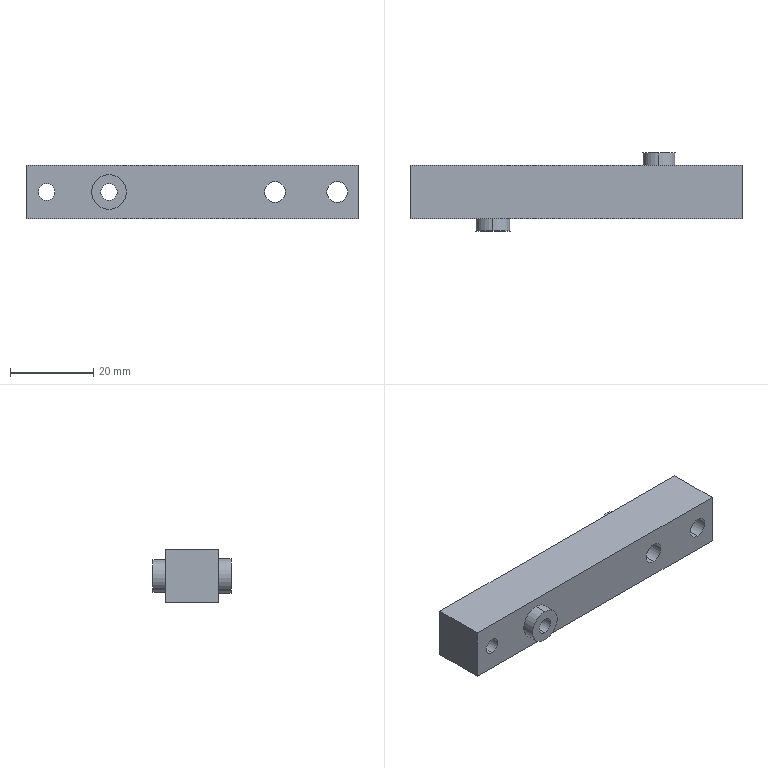Part | STEP file | Weighing module | 1 solid | 20 faces | box 80 x 18.8 x 12.8 mm | volume 12498 mm3 | cylinder 12 | plane 8 | commonest cylinder face diameters 4 x4 5 x4 7.89 x2 8.361 x2
STEP:
#1=CARTESIAN_POINT('',(0.,0.,0.));
#2=DIRECTION('',(0.,0.,1.));
#3=DIRECTION('',(1.,0.,0.));
#4=AXIS2_PLACEMENT_3D('',#1,#2,#3);
#5=CARTESIAN_POINT('',(20.,9.4,10.345));
#6=VERTEX_POINT('',#5);
#7=CARTESIAN_POINT('',(20.,9.4,2.455));
#8=VERTEX_POINT('',#7);
#9=CARTESIAN_POINT('',(20.,9.4,6.4));
#10=DIRECTION('',(0.,1.,0.));
#11=DIRECTION('',(0.,0.,1.));
#12=AXIS2_PLACEMENT_3D('',#9,#10,#11);
#13=CIRCLE('',#12,3.945);
#14=CARTESIAN_POINT('',(20.,9.4,6.4));
#15=DIRECTION('',(0.,-1.,0.));
#16=DIRECTION('',(0.,0.,-1.));
#17=AXIS2_PLACEMENT_3D('',#14,#15,#16);
#18=CYLINDRICAL_SURFACE('',#17,3.945);
#19=CARTESIAN_POINT('',(3.142,0.));
#20=DIRECTION('',(-1.,0.));
#21=VECTOR('',#20,1.);
#22=LINE('',#19,#21);
#23=(GEOMETRIC_REPRESENTATION_CONTEXT(2)PARAMETRIC_REPRESENTATION_CONTEXT()REPRESENTATION_CONTEXT('',''));
#24=DEFINITIONAL_REPRESENTATION('',(#22),#23);
#25=PCURVE('',#18,#24);
#26=CARTESIAN_POINT('',(20.,9.4,6.4));
#27=DIRECTION('',(0.,1.,0.));
#28=DIRECTION('',(0.,0.,1.));
#29=AXIS2_PLACEMENT_3D('',#26,#27,#28);
#30=PLANE('',#29);
#31=CARTESIAN_POINT('',(0.,0.));
#32=DIRECTION('',(1.,0.));
#33=AXIS2_PLACEMENT_2D('',#31,#32);
#34=CIRCLE('',#33,3.945);
#35=(GEOMETRIC_REPRESENTATION_CONTEXT(2)PARAMETRIC_REPRESENTATION_CONTEXT()REPRESENTATION_CONTEXT('',''));
#36=DEFINITIONAL_REPRESENTATION('',(#34),#35);
#37=PCURVE('',#30,#36);
#38=SURFACE_CURVE('',#13,(#25,#37),.PCURVE_S1.);
#39=EDGE_CURVE('',#6,#8,#38,.T.);
#40=ORIENTED_EDGE('',*,*,#39,.F.);
#41=CARTESIAN_POINT('',(20.,6.4,10.345));
#42=VERTEX_POINT('',#41);
#43=CARTESIAN_POINT('',(20.,9.4,10.345));
#44=DIRECTION('',(0.,-1.,0.));
#45=VECTOR('',#44,1.);
#46=LINE('',#43,#45);
#47=CARTESIAN_POINT('',(3.142,0.));
#48=DIRECTION('',(0.,1.));
#49=VECTOR('',#48,1.);
#50=LINE('',#47,#49);
#51=(GEOMETRIC_REPRESENTATION_CONTEXT(2)PARAMETRIC_REPRESENTATION_CONTEXT()REPRESENTATION_CONTEXT('',''));
#52=DEFINITIONAL_REPRESENTATION('',(#50),#51);
#53=PCURVE('',#18,#52);
#54=CARTESIAN_POINT('',(20.,9.4,6.4));
#55=DIRECTION('',(0.,-1.,0.));
#56=DIRECTION('',(0.,0.,-1.));
#57=AXIS2_PLACEMENT_3D('',#54,#55,#56);
#58=CYLINDRICAL_SURFACE('',#57,3.945);
#59=CARTESIAN_POINT('',(3.142,0.));
#60=DIRECTION('',(0.,1.));
#61=VECTOR('',#60,1.);
#62=LINE('',#59,#61);
#63=(GEOMETRIC_REPRESENTATION_CONTEXT(2)PARAMETRIC_REPRESENTATION_CONTEXT()REPRESENTATION_CONTEXT('',''));
#64=DEFINITIONAL_REPRESENTATION('',(#62),#63);
#65=PCURVE('',#58,#64);
#66=SURFACE_CURVE('',#46,(#53,#65),.PCURVE_S1.);
#67=EDGE_CURVE('',#6,#42,#66,.T.);
#68=ORIENTED_EDGE('',*,*,#67,.T.);
#69=CARTESIAN_POINT('',(20.,6.4,2.455));
#70=VERTEX_POINT('',#69);
#71=CARTESIAN_POINT('',(20.,6.4,6.4));
#72=DIRECTION('',(0.,1.,0.));
#73=DIRECTION('',(0.,0.,-1.));
#74=AXIS2_PLACEMENT_3D('',#71,#72,#73);
#75=CIRCLE('',#74,3.945);
#76=CARTESIAN_POINT('',(6.283,3.));
#77=DIRECTION('',(-1.,0.));
#78=VECTOR('',#77,1.);
#79=LINE('',#76,#78);
#80=(GEOMETRIC_REPRESENTATION_CONTEXT(2)PARAMETRIC_REPRESENTATION_CONTEXT()REPRESENTATION_CONTEXT('',''));
#81=DEFINITIONAL_REPRESENTATION('',(#79),#80);
#82=PCURVE('',#18,#81);
#83=CARTESIAN_POINT('',(-40.,6.4,12.8));
#84=DIRECTION('',(0.,-1.,0.));
#85=DIRECTION('',(0.,0.,-1.));
#86=AXIS2_PLACEMENT_3D('',#83,#84,#85);
#87=PLANE('',#86);
#88=CARTESIAN_POINT('',(10.345,60.));
#89=CARTESIAN_POINT('',(10.345,53.167));
#90=CARTESIAN_POINT('',(4.428,56.584));
#91=CARTESIAN_POINT('',(-1.49,60.));
#92=CARTESIAN_POINT('',(4.428,63.416));
#93=CARTESIAN_POINT('',(10.345,66.833));
#94=CARTESIAN_POINT('',(10.345,60.));
#95=(BOUNDED_CURVE()B_SPLINE_CURVE(2,(#88,#89,#90,#91,#92,#93,#94),.UNSPECIFIED.,.T.,.F.)B_SPLINE_CURVE_WITH_KNOTS((1,2,2,2,2,1),(-2.094,0.,2.094,4.189,6.283,8.378),.UNSPECIFIED.)CURVE()GEOMETRIC_REPRESENTATION_ITEM()RATIONAL_B_SPLINE_CURVE((1.,0.5,1.,0.5,1.,0.5,1.))REPRESENTATION_ITEM(''));
#96=(GEOMETRIC_REPRESENTATION_CONTEXT(2)PARAMETRIC_REPRESENTATION_CONTEXT()REPRESENTATION_CONTEXT('',''));
#97=DEFINITIONAL_REPRESENTATION('',(#95),#96);
#98=PCURVE('',#87,#97);
#99=SURFACE_CURVE('',#75,(#82,#98),.PCURVE_S1.);
#100=EDGE_CURVE('',#42,#70,#99,.T.);
#101=ORIENTED_EDGE('',*,*,#100,.T.);
#102=CARTESIAN_POINT('',(20.,9.4,2.455));
#103=DIRECTION('',(0.,-1.,0.));
#104=VECTOR('',#103,1.);
#105=LINE('',#102,#104);
#106=CARTESIAN_POINT('',(0.,0.));
#107=DIRECTION('',(0.,1.));
#108=VECTOR('',#107,1.);
#109=LINE('',#106,#108);
#110=(GEOMETRIC_REPRESENTATION_CONTEXT(2)PARAMETRIC_REPRESENTATION_CONTEXT()REPRESENTATION_CONTEXT('',''));
#111=DEFINITIONAL_REPRESENTATION('',(#109),#110);
#112=PCURVE('',#18,#111);
#113=CARTESIAN_POINT('',(6.283,0.));
#114=DIRECTION('',(0.,1.));
#115=VECTOR('',#114,1.);
#116=LINE('',#113,#115);
#117=(GEOMETRIC_REPRESENTATION_CONTEXT(2)PARAMETRIC_REPRESENTATION_CONTEXT()REPRESENTATION_CONTEXT('',''));
#118=DEFINITIONAL_REPRESENTATION('',(#116),#117);
#119=PCURVE('',#58,#118);
#120=SURFACE_CURVE('',#105,(#112,#119),.PCURVE_S1.);
#121=EDGE_CURVE('',#8,#70,#120,.T.);
#122=ORIENTED_EDGE('',*,*,#121,.F.);
#123=EDGE_LOOP('',(#40,#68,#101,#122));
#124=FACE_BOUND('',#123,.T.);
#125=ADVANCED_FACE('',(#124),#18,.T.);
#126=CARTESIAN_POINT('',(-20.,-9.4,2.22));
#127=VERTEX_POINT('',#126);
#128=CARTESIAN_POINT('',(-20.,-9.4,10.58));
#129=VERTEX_POINT('',#128);
#130=CARTESIAN_POINT('',(-20.,-9.4,6.4));
#131=DIRECTION('',(0.,-1.,0.));
#132=DIRECTION('',(0.,0.,-1.));
#133=AXIS2_PLACEMENT_3D('',#130,#131,#132);
#134=CIRCLE('',#133,4.18);
#135=CARTESIAN_POINT('',(-20.,-9.4,6.4));
#136=DIRECTION('',(0.,1.,0.));
#137=DIRECTION('',(0.,0.,1.));
#138=AXIS2_PLACEMENT_3D('',#135,#136,#137);
#139=CYLINDRICAL_SURFACE('',#138,4.18);
#140=CARTESIAN_POINT('',(3.142,0.));
#141=DIRECTION('',(-1.,0.));
#142=VECTOR('',#141,1.);
#143=LINE('',#140,#142);
#144=(GEOMETRIC_REPRESENTATION_CONTEXT(2)PARAMETRIC_REPRESENTATION_CONTEXT()REPRESENTATION_CONTEXT('',''));
#145=DEFINITIONAL_REPRESENTATION('',(#143),#144);
#146=PCURVE('',#139,#145);
#147=CARTESIAN_POINT('',(-20.,-9.4,6.4));
#148=DIRECTION('',(0.,-1.,0.));
#149=DIRECTION('',(0.,0.,-1.));
#150=AXIS2_PLACEMENT_3D('',#147,#148,#149);
#151=PLANE('',#150);
#152=CARTESIAN_POINT('',(0.,0.));
#153=DIRECTION('',(1.,0.));
#154=AXIS2_PLACEMENT_2D('',#152,#153);
#155=CIRCLE('',#154,4.18);
#156=(GEOMETRIC_REPRESENTATION_CONTEXT(2)PARAMETRIC_REPRESENTATION_CONTEXT()REPRESENTATION_CONTEXT('',''));
#157=DEFINITIONAL_REPRESENTATION('',(#155),#156);
#158=PCURVE('',#151,#157);
#159=SURFACE_CURVE('',#134,(#146,#158),.PCURVE_S1.);
#160=EDGE_CURVE('',#127,#129,#159,.T.);
#161=ORIENTED_EDGE('',*,*,#160,.F.);
#162=CARTESIAN_POINT('',(-20.,-6.4,2.22));
#163=VERTEX_POINT('',#162);
#164=CARTESIAN_POINT('',(-20.,-9.4,2.22));
#165=DIRECTION('',(0.,1.,0.));
#166=VECTOR('',#165,1.);
#167=LINE('',#164,#166);
#168=CARTESIAN_POINT('',(3.142,0.));
#169=DIRECTION('',(0.,1.));
#170=VECTOR('',#169,1.);
#171=LINE('',#168,#170);
#172=(GEOMETRIC_REPRESENTATION_CONTEXT(2)PARAMETRIC_REPRESENTATION_CONTEXT()REPRESENTATION_CONTEXT('',''));
#173=DEFINITIONAL_REPRESENTATION('',(#171),#172);
#174=PCURVE('',#139,#173);
#175=CARTESIAN_POINT('',(-20.,-9.4,6.4));
#176=DIRECTION('',(0.,1.,0.));
#177=DIRECTION('',(0.,0.,1.));
#178=AXIS2_PLACEMENT_3D('',#175,#176,#177);
#179=CYLINDRICAL_SURFACE('',#178,4.18);
#180=CARTESIAN_POINT('',(3.142,0.));
#181=DIRECTION('',(0.,1.));
#182=VECTOR('',#181,1.);
#183=LINE('',#180,#182);
#184=(GEOMETRIC_REPRESENTATION_CONTEXT(2)PARAMETRIC_REPRESENTATION_CONTEXT()REPRESENTATION_CONTEXT('',''));
#185=DEFINITIONAL_REPRESENTATION('',(#183),#184);
#186=PCURVE('',#179,#185);
#187=SURFACE_CURVE('',#167,(#174,#186),.PCURVE_S1.);
#188=EDGE_CURVE('',#127,#163,#187,.T.);
#189=ORIENTED_EDGE('',*,*,#188,.T.);
#190=CARTESIAN_POINT('',(-20.,-6.4,10.58));
#191=VERTEX_POINT('',#190);
#192=CARTESIAN_POINT('',(-20.,-6.4,6.4));
#193=DIRECTION('',(0.,-1.,0.));
#194=DIRECTION('',(0.,0.,1.));
#195=AXIS2_PLACEMENT_3D('',#192,#193,#194);
#196=CIRCLE('',#195,4.18);
#197=CARTESIAN_POINT('',(6.283,3.));
#198=DIRECTION('',(-1.,0.));
#199=VECTOR('',#198,1.);
#200=LINE('',#197,#199);
#201=(GEOMETRIC_REPRESENTATION_CONTEXT(2)PARAMETRIC_REPRESENTATION_CONTEXT()REPRESENTATION_CONTEXT('',''));
#202=DEFINITIONAL_REPRESENTATION('',(#200),#201);
#203=PCURVE('',#139,#202);
#204=CARTESIAN_POINT('',(-40.,-6.4,12.8));
#205=DIRECTION('',(0.,1.,0.));
#206=DIRECTION('',(0.,0.,1.));
#207=AXIS2_PLACEMENT_3D('',#204,#205,#206);
#208=PLANE('',#207);
#209=CARTESIAN_POINT('',(-2.22,20.));
#210=CARTESIAN_POINT('',(-2.22,12.759));
#211=CARTESIAN_POINT('',(-8.49,16.38));
#212=CARTESIAN_POINT('',(-14.761,20.));
#213=CARTESIAN_POINT('',(-8.49,23.62));
#214=CARTESIAN_POINT('',(-2.22,27.241));
#215=CARTESIAN_POINT('',(-2.22,20.));
#216=(BOUNDED_CURVE()B_SPLINE_CURVE(2,(#209,#210,#211,#212,#213,#214,#215),.UNSPECIFIED.,.T.,.F.)B_SPLINE_CURVE_WITH_KNOTS((1,2,2,2,2,1),(-2.094,0.,2.094,4.189,6.283,8.378),.UNSPECIFIED.)CURVE()GEOMETRIC_REPRESENTATION_ITEM()RATIONAL_B_SPLINE_CURVE((1.,0.5,1.,0.5,1.,0.5,1.))REPRESENTATION_ITEM(''));
#217=(GEOMETRIC_REPRESENTATION_CONTEXT(2)PARAMETRIC_REPRESENTATION_CONTEXT()REPRESENTATION_CONTEXT('',''));
#218=DEFINITIONAL_REPRESENTATION('',(#216),#217);
#219=PCURVE('',#208,#218);
#220=SURFACE_CURVE('',#196,(#203,#219),.PCURVE_S1.);
#221=EDGE_CURVE('',#163,#191,#220,.T.);
#222=ORIENTED_EDGE('',*,*,#221,.T.);
#223=CARTESIAN_POINT('',(-20.,-9.4,10.58));
#224=DIRECTION('',(0.,1.,0.));
#225=VECTOR('',#224,1.);
#226=LINE('',#223,#225);
#227=CARTESIAN_POINT('',(0.,0.));
#228=DIRECTION('',(0.,1.));
#229=VECTOR('',#228,1.);
#230=LINE('',#227,#229);
#231=(GEOMETRIC_REPRESENTATION_CONTEXT(2)PARAMETRIC_REPRESENTATION_CONTEXT()REPRESENTATION_CONTEXT('',''));
#232=DEFINITIONAL_REPRESENTATION('',(#230),#231);
#233=PCURVE('',#139,#232);
#234=CARTESIAN_POINT('',(6.283,0.));
#235=DIRECTION('',(0.,1.));
#236=VECTOR('',#235,1.);
#237=LINE('',#234,#236);
#238=(GEOMETRIC_REPRESENTATION_CONTEXT(2)PARAMETRIC_REPRESENTATION_CONTEXT()REPRESENTATION_CONTEXT('',''));
#239=DEFINITIONAL_REPRESENTATION('',(#237),#238);
#240=PCURVE('',#179,#239);
#241=SURFACE_CURVE('',#226,(#233,#240),.PCURVE_S1.);
#242=EDGE_CURVE('',#129,#191,#241,.T.);
#243=ORIENTED_EDGE('',*,*,#242,.F.);
#244=EDGE_LOOP('',(#161,#189,#222,#243));
#245=FACE_BOUND('',#244,.T.);
#246=ADVANCED_FACE('',(#245),#139,.T.);
#247=CARTESIAN_POINT('',(-35.,-6.4,8.4));
#248=VERTEX_POINT('',#247);
#249=CARTESIAN_POINT('',(-35.,6.4,8.4));
#250=VERTEX_POINT('',#249);
#251=CARTESIAN_POINT('',(-35.,-6.4,8.4));
#252=DIRECTION('',(0.,1.,0.));
#253=VECTOR('',#252,1.);
#254=LINE('',#251,#253);
#255=CARTESIAN_POINT('',(-35.,-6.4,6.4));
#256=DIRECTION('',(0.,1.,0.));
#257=DIRECTION('',(0.,0.,1.));
#258=AXIS2_PLACEMENT_3D('',#255,#256,#257);
#259=CYLINDRICAL_SURFACE('',#258,2.);
#260=CARTESIAN_POINT('',(6.283,0.));
#261=DIRECTION('',(0.,1.));
#262=VECTOR('',#261,1.);
#263=LINE('',#260,#262);
#264=(GEOMETRIC_REPRESENTATION_CONTEXT(2)PARAMETRIC_REPRESENTATION_CONTEXT()REPRESENTATION_CONTEXT('',''));
#265=DEFINITIONAL_REPRESENTATION('',(#263),#264);
#266=PCURVE('',#259,#265);
#267=CARTESIAN_POINT('',(-35.,-6.4,6.4));
#268=DIRECTION('',(0.,1.,0.));
#269=DIRECTION('',(0.,0.,1.));
#270=AXIS2_PLACEMENT_3D('',#267,#268,#269);
#271=CYLINDRICAL_SURFACE('',#270,2.);
#272=CARTESIAN_POINT('',(0.,0.));
#273=DIRECTION('',(0.,1.));
#274=VECTOR('',#273,1.);
#275=LINE('',#272,#274);
#276=(GEOMETRIC_REPRESENTATION_CONTEXT(2)PARAMETRIC_REPRESENTATION_CONTEXT()REPRESENTATION_CONTEXT('',''));
#277=DEFINITIONAL_REPRESENTATION('',(#275),#276);
#278=PCURVE('',#271,#277);
#279=SURFACE_CURVE('',#254,(#266,#278),.PCURVE_S1.);
#280=EDGE_CURVE('',#248,#250,#279,.T.);
#281=ORIENTED_EDGE('',*,*,#280,.T.);
#282=CARTESIAN_POINT('',(-35.,6.4,4.4));
#283=VERTEX_POINT('',#282);
#284=CARTESIAN_POINT('',(-35.,6.4,6.4));
#285=DIRECTION('',(0.,1.,0.));
#286=DIRECTION('',(0.,0.,1.));
#287=AXIS2_PLACEMENT_3D('',#284,#285,#286);
#288=CIRCLE('',#287,2.);
#289=CARTESIAN_POINT('',(0.,12.8));
#290=DIRECTION('',(1.,0.));
#291=VECTOR('',#290,1.);
#292=LINE('',#289,#291);
#293=(GEOMETRIC_REPRESENTATION_CONTEXT(2)PARAMETRIC_REPRESENTATION_CONTEXT()REPRESENTATION_CONTEXT('',''));
#294=DEFINITIONAL_REPRESENTATION('',(#292),#293);
#295=PCURVE('',#259,#294);
#296=CARTESIAN_POINT('',(4.4,5.));
#297=CARTESIAN_POINT('',(4.4,8.464));
#298=CARTESIAN_POINT('',(7.4,6.732));
#299=CARTESIAN_POINT('',(10.4,5.));
#300=CARTESIAN_POINT('',(7.4,3.268));
#301=CARTESIAN_POINT('',(4.4,1.536));
#302=CARTESIAN_POINT('',(4.4,5.));
#303=(BOUNDED_CURVE()B_SPLINE_CURVE(2,(#296,#297,#298,#299,#300,#301,#302),.UNSPECIFIED.,.T.,.F.)B_SPLINE_CURVE_WITH_KNOTS((1,2,2,2,2,1),(-2.094,0.,2.094,4.189,6.283,8.378),.UNSPECIFIED.)CURVE()GEOMETRIC_REPRESENTATION_ITEM()RATIONAL_B_SPLINE_CURVE((1.,0.5,1.,0.5,1.,0.5,1.))REPRESENTATION_ITEM(''));
#304=(GEOMETRIC_REPRESENTATION_CONTEXT(2)PARAMETRIC_REPRESENTATION_CONTEXT()REPRESENTATION_CONTEXT('',''));
#305=DEFINITIONAL_REPRESENTATION('',(#303),#304);
#306=PCURVE('',#87,#305);
#307=SURFACE_CURVE('',#288,(#295,#306),.PCURVE_S1.);
#308=EDGE_CURVE('',#283,#250,#307,.T.);
#309=ORIENTED_EDGE('',*,*,#308,.F.);
#310=CARTESIAN_POINT('',(-35.,-6.4,4.4));
#311=VERTEX_POINT('',#310);
#312=CARTESIAN_POINT('',(-35.,-6.4,4.4));
#313=DIRECTION('',(0.,1.,0.));
#314=VECTOR('',#313,1.);
#315=LINE('',#312,#314);
#316=CARTESIAN_POINT('',(3.142,0.));
#317=DIRECTION('',(0.,1.));
#318=VECTOR('',#317,1.);
#319=LINE('',#316,#318);
#320=(GEOMETRIC_REPRESENTATION_CONTEXT(2)PARAMETRIC_REPRESENTATION_CONTEXT()REPRESENTATION_CONTEXT('',''));
#321=DEFINITIONAL_REPRESENTATION('',(#319),#320);
#322=PCURVE('',#259,#321);
#323=CARTESIAN_POINT('',(3.142,0.));
#324=DIRECTION('',(0.,1.));
#325=VECTOR('',#324,1.);
#326=LINE('',#323,#325);
#327=(GEOMETRIC_REPRESENTATION_CONTEXT(2)PARAMETRIC_REPRESENTATION_CONTEXT()REPRESENTATION_CONTEXT('',''));
#328=DEFINITIONAL_REPRESENTATION('',(#326),#327);
#329=PCURVE('',#271,#328);
#330=SURFACE_CURVE('',#315,(#322,#329),.PCURVE_S1.);
#331=EDGE_CURVE('',#311,#283,#330,.T.);
#332=ORIENTED_EDGE('',*,*,#331,.F.);
#333=CARTESIAN_POINT('',(-35.,-6.4,6.4));
#334=DIRECTION('',(0.,1.,0.));
#335=DIRECTION('',(0.,0.,1.));
#336=AXIS2_PLACEMENT_3D('',#333,#334,#335);
#337=CIRCLE('',#336,2.);
#338=CARTESIAN_POINT('',(0.,0.));
#339=DIRECTION('',(1.,0.));
#340=VECTOR('',#339,1.);
#341=LINE('',#338,#340);
#342=(GEOMETRIC_REPRESENTATION_CONTEXT(2)PARAMETRIC_REPRESENTATION_CONTEXT()REPRESENTATION_CONTEXT('',''));
#343=DEFINITIONAL_REPRESENTATION('',(#341),#342);
#344=PCURVE('',#259,#343);
#345=CARTESIAN_POINT('',(-6.4,5.));
#346=DIRECTION('',(1.,0.));
#347=AXIS2_PLACEMENT_2D('',#345,#346);
#348=CIRCLE('',#347,2.);
#349=(GEOMETRIC_REPRESENTATION_CONTEXT(2)PARAMETRIC_REPRESENTATION_CONTEXT()REPRESENTATION_CONTEXT('',''));
#350=DEFINITIONAL_REPRESENTATION('',(#348),#349);
#351=PCURVE('',#208,#350);
#352=SURFACE_CURVE('',#337,(#344,#351),.PCURVE_S1.);
#353=EDGE_CURVE('',#311,#248,#352,.T.);
#354=ORIENTED_EDGE('',*,*,#353,.T.);
#355=EDGE_LOOP('',(#281,#309,#332,#354));
#356=FACE_BOUND('',#355,.F.);
#357=ADVANCED_FACE('',(#356),#259,.F.);
#358=CARTESIAN_POINT('',(-20.,-9.4,8.4));
#359=VERTEX_POINT('',#358);
#360=CARTESIAN_POINT('',(-20.,6.4,8.4));
#361=VERTEX_POINT('',#360);
#362=CARTESIAN_POINT('',(-20.,-6.4,8.4));
#363=DIRECTION('',(0.,1.,0.));
#364=VECTOR('',#363,1.);
#365=LINE('',#362,#364);
#366=CARTESIAN_POINT('',(-20.,-6.4,6.4));
#367=DIRECTION('',(0.,1.,0.));
#368=DIRECTION('',(0.,0.,1.));
#369=AXIS2_PLACEMENT_3D('',#366,#367,#368);
#370=CYLINDRICAL_SURFACE('',#369,2.);
#371=CARTESIAN_POINT('',(6.283,0.));
#372=DIRECTION('',(0.,1.));
#373=VECTOR('',#372,1.);
#374=LINE('',#371,#373);
#375=(GEOMETRIC_REPRESENTATION_CONTEXT(2)PARAMETRIC_REPRESENTATION_CONTEXT()REPRESENTATION_CONTEXT('',''));
#376=DEFINITIONAL_REPRESENTATION('',(#374),#375);
#377=PCURVE('',#370,#376);
#378=CARTESIAN_POINT('',(-20.,-6.4,6.4));
#379=DIRECTION('',(0.,1.,0.));
#380=DIRECTION('',(0.,0.,1.));
#381=AXIS2_PLACEMENT_3D('',#378,#379,#380);
#382=CYLINDRICAL_SURFACE('',#381,2.);
#383=CARTESIAN_POINT('',(0.,0.));
#384=DIRECTION('',(0.,1.));
#385=VECTOR('',#384,1.);
#386=LINE('',#383,#385);
#387=(GEOMETRIC_REPRESENTATION_CONTEXT(2)PARAMETRIC_REPRESENTATION_CONTEXT()REPRESENTATION_CONTEXT('',''));
#388=DEFINITIONAL_REPRESENTATION('',(#386),#387);
#389=PCURVE('',#382,#388);
#390=SURFACE_CURVE('',#365,(#377,#389),.PCURVE_S1.);
#391=EDGE_CURVE('',#359,#361,#390,.T.);
#392=ORIENTED_EDGE('',*,*,#391,.T.);
#393=CARTESIAN_POINT('',(-20.,6.4,4.4));
#394=VERTEX_POINT('',#393);
#395=CARTESIAN_POINT('',(-20.,6.4,6.4));
#396=DIRECTION('',(0.,1.,0.));
#397=DIRECTION('',(0.,0.,1.));
#398=AXIS2_PLACEMENT_3D('',#395,#396,#397);
#399=CIRCLE('',#398,2.);
#400=CARTESIAN_POINT('',(0.,12.8));
#401=DIRECTION('',(1.,0.));
#402=VECTOR('',#401,1.);
#403=LINE('',#400,#402);
#404=(GEOMETRIC_REPRESENTATION_CONTEXT(2)PARAMETRIC_REPRESENTATION_CONTEXT()REPRESENTATION_CONTEXT('',''));
#405=DEFINITIONAL_REPRESENTATION('',(#403),#404);
#406=PCURVE('',#370,#405);
#407=CARTESIAN_POINT('',(4.4,20.));
#408=CARTESIAN_POINT('',(4.4,23.464));
#409=CARTESIAN_POINT('',(7.4,21.732));
#410=CARTESIAN_POINT('',(10.4,20.));
#411=CARTESIAN_POINT('',(7.4,18.268));
#412=CARTESIAN_POINT('',(4.4,16.536));
#413=CARTESIAN_POINT('',(4.4,20.));
#414=(BOUNDED_CURVE()B_SPLINE_CURVE(2,(#407,#408,#409,#410,#411,#412,#413),.UNSPECIFIED.,.T.,.F.)B_SPLINE_CURVE_WITH_KNOTS((1,2,2,2,2,1),(-2.094,0.,2.094,4.189,6.283,8.378),.UNSPECIFIED.)CURVE()GEOMETRIC_REPRESENTATION_ITEM()RATIONAL_B_SPLINE_CURVE((1.,0.5,1.,0.5,1.,0.5,1.))REPRESENTATION_ITEM(''));
#415=(GEOMETRIC_REPRESENTATION_CONTEXT(2)PARAMETRIC_REPRESENTATION_CONTEXT()REPRESENTATION_CONTEXT('',''));
#416=DEFINITIONAL_REPRESENTATION('',(#414),#415);
#417=PCURVE('',#87,#416);
#418=SURFACE_CURVE('',#399,(#406,#417),.PCURVE_S1.);
#419=EDGE_CURVE('',#394,#361,#418,.T.);
#420=ORIENTED_EDGE('',*,*,#419,.F.);
#421=CARTESIAN_POINT('',(-20.,-9.4,4.4));
#422=VERTEX_POINT('',#421);
#423=CARTESIAN_POINT('',(-20.,-6.4,4.4));
#424=DIRECTION('',(0.,1.,0.));
#425=VECTOR('',#424,1.);
#426=LINE('',#423,#425);
#427=CARTESIAN_POINT('',(3.142,0.));
#428=DIRECTION('',(0.,1.));
#429=VECTOR('',#428,1.);
#430=LINE('',#427,#429);
#431=(GEOMETRIC_REPRESENTATION_CONTEXT(2)PARAMETRIC_REPRESENTATION_CONTEXT()REPRESENTATION_CONTEXT('',''));
#432=DEFINITIONAL_REPRESENTATION('',(#430),#431);
#433=PCURVE('',#370,#432);
#434=CARTESIAN_POINT('',(3.142,0.));
#435=DIRECTION('',(0.,1.));
#436=VECTOR('',#435,1.);
#437=LINE('',#434,#436);
#438=(GEOMETRIC_REPRESENTATION_CONTEXT(2)PARAMETRIC_REPRESENTATION_CONTEXT()REPRESENTATION_CONTEXT('',''));
#439=DEFINITIONAL_REPRESENTATION('',(#437),#438);
#440=PCURVE('',#382,#439);
#441=SURFACE_CURVE('',#426,(#433,#440),.PCURVE_S1.);
#442=EDGE_CURVE('',#422,#394,#441,.T.);
#443=ORIENTED_EDGE('',*,*,#442,.F.);
#444=CARTESIAN_POINT('',(-20.,-9.4,6.4));
#445=DIRECTION('',(0.,-1.,0.));
#446=DIRECTION('',(0.,0.,-1.));
#447=AXIS2_PLACEMENT_3D('',#444,#445,#446);
#448=CIRCLE('',#447,2.);
#449=CARTESIAN_POINT('',(9.425,-3.));
#450=DIRECTION('',(-1.,0.));
#451=VECTOR('',#450,1.);
#452=LINE('',#449,#451);
#453=(GEOMETRIC_REPRESENTATION_CONTEXT(2)PARAMETRIC_REPRESENTATION_CONTEXT()REPRESENTATION_CONTEXT('',''));
#454=DEFINITIONAL_REPRESENTATION('',(#452),#453);
#455=PCURVE('',#370,#454);
#456=CARTESIAN_POINT('',(0.,0.));
#457=DIRECTION('',(1.,0.));
#458=AXIS2_PLACEMENT_2D('',#456,#457);
#459=CIRCLE('',#458,2.);
#460=(GEOMETRIC_REPRESENTATION_CONTEXT(2)PARAMETRIC_REPRESENTATION_CONTEXT()REPRESENTATION_CONTEXT('',''));
#461=DEFINITIONAL_REPRESENTATION('',(#459),#460);
#462=PCURVE('',#151,#461);
#463=SURFACE_CURVE('',#448,(#455,#462),.PCURVE_S1.);
#464=EDGE_CURVE('',#359,#422,#463,.T.);
#465=ORIENTED_EDGE('',*,*,#464,.F.);
#466=EDGE_LOOP('',(#392,#420,#443,#465));
#467=FACE_BOUND('',#466,.F.);
#468=ADVANCED_FACE('',(#467),#370,.F.);
#469=CARTESIAN_POINT('',(35.,-6.4,8.9));
#470=VERTEX_POINT('',#469);
#471=CARTESIAN_POINT('',(35.,6.4,8.9));
#472=VERTEX_POINT('',#471);
#473=CARTESIAN_POINT('',(35.,-6.4,8.9));
#474=DIRECTION('',(0.,1.,0.));
#475=VECTOR('',#474,1.);
#476=LINE('',#473,#475);
#477=CARTESIAN_POINT('',(35.,-6.4,6.4));
#478=DIRECTION('',(0.,1.,0.));
#479=DIRECTION('',(0.,0.,1.));
#480=AXIS2_PLACEMENT_3D('',#477,#478,#479);
#481=CYLINDRICAL_SURFACE('',#480,2.5);
#482=CARTESIAN_POINT('',(6.283,0.));
#483=DIRECTION('',(0.,1.));
#484=VECTOR('',#483,1.);
#485=LINE('',#482,#484);
#486=(GEOMETRIC_REPRESENTATION_CONTEXT(2)PARAMETRIC_REPRESENTATION_CONTEXT()REPRESENTATION_CONTEXT('',''));
#487=DEFINITIONAL_REPRESENTATION('',(#485),#486);
#488=PCURVE('',#481,#487);
#489=CARTESIAN_POINT('',(35.,-6.4,6.4));
#490=DIRECTION('',(0.,1.,0.));
#491=DIRECTION('',(0.,0.,1.));
#492=AXIS2_PLACEMENT_3D('',#489,#490,#491);
#493=CYLINDRICAL_SURFACE('',#492,2.5);
#494=CARTESIAN_POINT('',(0.,0.));
#495=DIRECTION('',(0.,1.));
#496=VECTOR('',#495,1.);
#497=LINE('',#494,#496);
#498=(GEOMETRIC_REPRESENTATION_CONTEXT(2)PARAMETRIC_REPRESENTATION_CONTEXT()REPRESENTATION_CONTEXT('',''));
#499=DEFINITIONAL_REPRESENTATION('',(#497),#498);
#500=PCURVE('',#493,#499);
#501=SURFACE_CURVE('',#476,(#488,#500),.PCURVE_S1.);
#502=EDGE_CURVE('',#470,#472,#501,.T.);
#503=ORIENTED_EDGE('',*,*,#502,.T.);
#504=CARTESIAN_POINT('',(35.,6.4,3.9));
#505=VERTEX_POINT('',#504);
#506=CARTESIAN_POINT('',(35.,6.4,6.4));
#507=DIRECTION('',(0.,1.,0.));
#508=DIRECTION('',(0.,0.,1.));
#509=AXIS2_PLACEMENT_3D('',#506,#507,#508);
#510=CIRCLE('',#509,2.5);
#511=CARTESIAN_POINT('',(0.,12.8));
#512=DIRECTION('',(1.,0.));
#513=VECTOR('',#512,1.);
#514=LINE('',#511,#513);
#515=(GEOMETRIC_REPRESENTATION_CONTEXT(2)PARAMETRIC_REPRESENTATION_CONTEXT()REPRESENTATION_CONTEXT('',''));
#516=DEFINITIONAL_REPRESENTATION('',(#514),#515);
#517=PCURVE('',#481,#516);
#518=CARTESIAN_POINT('',(3.9,75.));
#519=CARTESIAN_POINT('',(3.9,79.33));
#520=CARTESIAN_POINT('',(7.65,77.165));
#521=CARTESIAN_POINT('',(11.4,75.));
#522=CARTESIAN_POINT('',(7.65,72.835));
#523=CARTESIAN_POINT('',(3.9,70.67));
#524=CARTESIAN_POINT('',(3.9,75.));
#525=(BOUNDED_CURVE()B_SPLINE_CURVE(2,(#518,#519,#520,#521,#522,#523,#524),.UNSPECIFIED.,.T.,.F.)B_SPLINE_CURVE_WITH_KNOTS((1,2,2,2,2,1),(-2.094,0.,2.094,4.189,6.283,8.378),.UNSPECIFIED.)CURVE()GEOMETRIC_REPRESENTATION_ITEM()RATIONAL_B_SPLINE_CURVE((1.,0.5,1.,0.5,1.,0.5,1.))REPRESENTATION_ITEM(''));
#526=(GEOMETRIC_REPRESENTATION_CONTEXT(2)PARAMETRIC_REPRESENTATION_CONTEXT()REPRESENTATION_CONTEXT('',''));
#527=DEFINITIONAL_REPRESENTATION('',(#525),#526);
#528=PCURVE('',#87,#527);
#529=SURFACE_CURVE('',#510,(#517,#528),.PCURVE_S1.);
#530=EDGE_CURVE('',#505,#472,#529,.T.);
#531=ORIENTED_EDGE('',*,*,#530,.F.);
#532=CARTESIAN_POINT('',(35.,-6.4,3.9));
#533=VERTEX_POINT('',#532);
#534=CARTESIAN_POINT('',(35.,-6.4,3.9));
#535=DIRECTION('',(0.,1.,0.));
#536=VECTOR('',#535,1.);
#537=LINE('',#534,#536);
#538=CARTESIAN_POINT('',(3.142,0.));
#539=DIRECTION('',(0.,1.));
#540=VECTOR('',#539,1.);
#541=LINE('',#538,#540);
#542=(GEOMETRIC_REPRESENTATION_CONTEXT(2)PARAMETRIC_REPRESENTATION_CONTEXT()REPRESENTATION_CONTEXT('',''));
#543=DEFINITIONAL_REPRESENTATION('',(#541),#542);
#544=PCURVE('',#481,#543);
#545=CARTESIAN_POINT('',(3.142,0.));
#546=DIRECTION('',(0.,1.));
#547=VECTOR('',#546,1.);
#548=LINE('',#545,#547);
#549=(GEOMETRIC_REPRESENTATION_CONTEXT(2)PARAMETRIC_REPRESENTATION_CONTEXT()REPRESENTATION_CONTEXT('',''));
#550=DEFINITIONAL_REPRESENTATION('',(#548),#549);
#551=PCURVE('',#493,#550);
#552=SURFACE_CURVE('',#537,(#544,#551),.PCURVE_S1.);
#553=EDGE_CURVE('',#533,#505,#552,.T.);
#554=ORIENTED_EDGE('',*,*,#553,.F.);
#555=CARTESIAN_POINT('',(35.,-6.4,6.4));
#556=DIRECTION('',(0.,1.,0.));
#557=DIRECTION('',(0.,0.,1.));
#558=AXIS2_PLACEMENT_3D('',#555,#556,#557);
#559=CIRCLE('',#558,2.5);
#560=CARTESIAN_POINT('',(0.,0.));
#561=DIRECTION('',(1.,0.));
#562=VECTOR('',#561,1.);
#563=LINE('',#560,#562);
#564=(GEOMETRIC_REPRESENTATION_CONTEXT(2)PARAMETRIC_REPRESENTATION_CONTEXT()REPRESENTATION_CONTEXT('',''));
#565=DEFINITIONAL_REPRESENTATION('',(#563),#564);
#566=PCURVE('',#481,#565);
#567=CARTESIAN_POINT('',(-6.4,75.));
#568=DIRECTION('',(1.,0.));
#569=AXIS2_PLACEMENT_2D('',#567,#568);
#570=CIRCLE('',#569,2.5);
#571=(GEOMETRIC_REPRESENTATION_CONTEXT(2)PARAMETRIC_REPRESENTATION_CONTEXT()REPRESENTATION_CONTEXT('',''));
#572=DEFINITIONAL_REPRESENTATION('',(#570),#571);
#573=PCURVE('',#208,#572);
#574=SURFACE_CURVE('',#559,(#566,#573),.PCURVE_S1.);
#575=EDGE_CURVE('',#533,#470,#574,.T.);
#576=ORIENTED_EDGE('',*,*,#575,.T.);
#577=EDGE_LOOP('',(#503,#531,#554,#576));
#578=FACE_BOUND('',#577,.F.);
#579=ADVANCED_FACE('',(#578),#481,.F.);
#580=CARTESIAN_POINT('',(20.,-6.4,8.9));
#581=VERTEX_POINT('',#580);
#582=CARTESIAN_POINT('',(20.,9.4,8.9));
#583=VERTEX_POINT('',#582);
#584=CARTESIAN_POINT('',(20.,-6.4,8.9));
#585=DIRECTION('',(0.,1.,0.));
#586=VECTOR('',#585,1.);
#587=LINE('',#584,#586);
#588=CARTESIAN_POINT('',(20.,-6.4,6.4));
#589=DIRECTION('',(0.,1.,0.));
#590=DIRECTION('',(0.,0.,1.));
#591=AXIS2_PLACEMENT_3D('',#588,#589,#590);
#592=CYLINDRICAL_SURFACE('',#591,2.5);
#593=CARTESIAN_POINT('',(6.283,0.));
#594=DIRECTION('',(0.,1.));
#595=VECTOR('',#594,1.);
#596=LINE('',#593,#595);
#597=(GEOMETRIC_REPRESENTATION_CONTEXT(2)PARAMETRIC_REPRESENTATION_CONTEXT()REPRESENTATION_CONTEXT('',''));
#598=DEFINITIONAL_REPRESENTATION('',(#596),#597);
#599=PCURVE('',#592,#598);
#600=CARTESIAN_POINT('',(20.,-6.4,6.4));
#601=DIRECTION('',(0.,1.,0.));
#602=DIRECTION('',(0.,0.,1.));
#603=AXIS2_PLACEMENT_3D('',#600,#601,#602);
#604=CYLINDRICAL_SURFACE('',#603,2.5);
#605=CARTESIAN_POINT('',(0.,0.));
#606=DIRECTION('',(0.,1.));
#607=VECTOR('',#606,1.);
#608=LINE('',#605,#607);
#609=(GEOMETRIC_REPRESENTATION_CONTEXT(2)PARAMETRIC_REPRESENTATION_CONTEXT()REPRESENTATION_CONTEXT('',''));
#610=DEFINITIONAL_REPRESENTATION('',(#608),#609);
#611=PCURVE('',#604,#610);
#612=SURFACE_CURVE('',#587,(#599,#611),.PCURVE_S1.);
#613=EDGE_CURVE('',#581,#583,#612,.T.);
#614=ORIENTED_EDGE('',*,*,#613,.T.);
#615=CARTESIAN_POINT('',(20.,9.4,3.9));
#616=VERTEX_POINT('',#615);
#617=CARTESIAN_POINT('',(20.,9.4,6.4));
#618=DIRECTION('',(0.,1.,0.));
#619=DIRECTION('',(0.,0.,1.));
#620=AXIS2_PLACEMENT_3D('',#617,#618,#619);
#621=CIRCLE('',#620,2.5);
#622=CARTESIAN_POINT('',(0.,15.8));
#623=DIRECTION('',(1.,0.));
#624=VECTOR('',#623,1.);
#625=LINE('',#622,#624);
#626=(GEOMETRIC_REPRESENTATION_CONTEXT(2)PARAMETRIC_REPRESENTATION_CONTEXT()REPRESENTATION_CONTEXT('',''));
#627=DEFINITIONAL_REPRESENTATION('',(#625),#626);
#628=PCURVE('',#592,#627);
#629=CARTESIAN_POINT('',(0.,0.));
#630=DIRECTION('',(1.,0.));
#631=AXIS2_PLACEMENT_2D('',#629,#630);
#632=CIRCLE('',#631,2.5);
#633=(GEOMETRIC_REPRESENTATION_CONTEXT(2)PARAMETRIC_REPRESENTATION_CONTEXT()REPRESENTATION_CONTEXT('',''));
#634=DEFINITIONAL_REPRESENTATION('',(#632),#633);
#635=PCURVE('',#30,#634);
#636=SURFACE_CURVE('',#621,(#628,#635),.PCURVE_S1.);
#637=EDGE_CURVE('',#616,#583,#636,.T.);
#638=ORIENTED_EDGE('',*,*,#637,.F.);
#639=CARTESIAN_POINT('',(20.,-6.4,3.9));
#640=VERTEX_POINT('',#639);
#641=CARTESIAN_POINT('',(20.,-6.4,3.9));
#642=DIRECTION('',(0.,1.,0.));
#643=VECTOR('',#642,1.);
#644=LINE('',#641,#643);
#645=CARTESIAN_POINT('',(3.142,0.));
#646=DIRECTION('',(0.,1.));
#647=VECTOR('',#646,1.);
#648=LINE('',#645,#647);
#649=(GEOMETRIC_REPRESENTATION_CONTEXT(2)PARAMETRIC_REPRESENTATION_CONTEXT()REPRESENTATION_CONTEXT('',''));
#650=DEFINITIONAL_REPRESENTATION('',(#648),#649);
#651=PCURVE('',#592,#650);
#652=CARTESIAN_POINT('',(3.142,0.));
#653=DIRECTION('',(0.,1.));
#654=VECTOR('',#653,1.);
#655=LINE('',#652,#654);
#656=(GEOMETRIC_REPRESENTATION_CONTEXT(2)PARAMETRIC_REPRESENTATION_CONTEXT()REPRESENTATION_CONTEXT('',''));
#657=DEFINITIONAL_REPRESENTATION('',(#655),#656);
#658=PCURVE('',#604,#657);
#659=SURFACE_CURVE('',#644,(#651,#658),.PCURVE_S1.);
#660=EDGE_CURVE('',#640,#616,#659,.T.);
#661=ORIENTED_EDGE('',*,*,#660,.F.);
#662=CARTESIAN_POINT('',(20.,-6.4,6.4));
#663=DIRECTION('',(0.,1.,0.));
#664=DIRECTION('',(0.,0.,1.));
#665=AXIS2_PLACEMENT_3D('',#662,#663,#664);
#666=CIRCLE('',#665,2.5);
#667=CARTESIAN_POINT('',(0.,0.));
#668=DIRECTION('',(1.,0.));
#669=VECTOR('',#668,1.);
#670=LINE('',#667,#669);
#671=(GEOMETRIC_REPRESENTATION_CONTEXT(2)PARAMETRIC_REPRESENTATION_CONTEXT()REPRESENTATION_CONTEXT('',''));
#672=DEFINITIONAL_REPRESENTATION('',(#670),#671);
#673=PCURVE('',#592,#672);
#674=CARTESIAN_POINT('',(-6.4,60.));
#675=DIRECTION('',(1.,0.));
#676=AXIS2_PLACEMENT_2D('',#674,#675);
#677=CIRCLE('',#676,2.5);
#678=(GEOMETRIC_REPRESENTATION_CONTEXT(2)PARAMETRIC_REPRESENTATION_CONTEXT()REPRESENTATION_CONTEXT('',''));
#679=DEFINITIONAL_REPRESENTATION('',(#677),#678);
#680=PCURVE('',#208,#679);
#681=SURFACE_CURVE('',#666,(#673,#680),.PCURVE_S1.);
#682=EDGE_CURVE('',#640,#581,#681,.T.);
#683=ORIENTED_EDGE('',*,*,#682,.T.);
#684=EDGE_LOOP('',(#614,#638,#661,#683));
#685=FACE_BOUND('',#684,.F.);
#686=ADVANCED_FACE('',(#685),#592,.F.);
#687=CARTESIAN_POINT('',(40.,6.4,0.));
#688=VERTEX_POINT('',#687);
#689=CARTESIAN_POINT('',(-40.,6.4,0.));
#690=VERTEX_POINT('',#689);
#691=CARTESIAN_POINT('',(-40.,6.4,0.));
#692=DIRECTION('',(-1.,0.,0.));
#693=VECTOR('',#692,1.);
#694=LINE('',#691,#693);
#695=CARTESIAN_POINT('',(12.8,0.));
#696=DIRECTION('',(0.,-1.));
#697=VECTOR('',#696,1.);
#698=LINE('',#695,#697);
#699=(GEOMETRIC_REPRESENTATION_CONTEXT(2)PARAMETRIC_REPRESENTATION_CONTEXT()REPRESENTATION_CONTEXT('',''));
#700=DEFINITIONAL_REPRESENTATION('',(#698),#699);
#701=PCURVE('',#87,#700);
#702=CARTESIAN_POINT('',(0.,0.,0.));
#703=DIRECTION('',(0.,0.,-1.));
#704=DIRECTION('',(-1.,0.,0.));
#705=AXIS2_PLACEMENT_3D('',#702,#703,#704);
#706=PLANE('',#705);
#707=CARTESIAN_POINT('',(40.,6.4));
#708=DIRECTION('',(1.,0.));
#709=VECTOR('',#708,1.);
#710=LINE('',#707,#709);
#711=(GEOMETRIC_REPRESENTATION_CONTEXT(2)PARAMETRIC_REPRESENTATION_CONTEXT()REPRESENTATION_CONTEXT('',''));
#712=DEFINITIONAL_REPRESENTATION('',(#710),#711);
#713=PCURVE('',#706,#712);
#714=SURFACE_CURVE('',#694,(#701,#713),.PCURVE_S1.);
#715=EDGE_CURVE('',#688,#690,#714,.T.);
#716=ORIENTED_EDGE('',*,*,#715,.T.);
#717=CARTESIAN_POINT('',(-40.,6.4,12.8));
#718=VERTEX_POINT('',#717);
#719=CARTESIAN_POINT('',(-40.,6.4,12.8));
#720=DIRECTION('',(0.,0.,-1.));
#721=VECTOR('',#720,1.);
#722=LINE('',#719,#721);
#723=CARTESIAN_POINT('',(0.,0.));
#724=DIRECTION('',(1.,0.));
#725=VECTOR('',#724,1.);
#726=LINE('',#723,#725);
#727=(GEOMETRIC_REPRESENTATION_CONTEXT(2)PARAMETRIC_REPRESENTATION_CONTEXT()REPRESENTATION_CONTEXT('',''));
#728=DEFINITIONAL_REPRESENTATION('',(#726),#727);
#729=PCURVE('',#87,#728);
#730=CARTESIAN_POINT('',(-40.,-6.4,12.8));
#731=DIRECTION('',(1.,0.,0.));
#732=DIRECTION('',(0.,0.,-1.));
#733=AXIS2_PLACEMENT_3D('',#730,#731,#732);
#734=PLANE('',#733);
#735=CARTESIAN_POINT('',(0.,12.8));
#736=DIRECTION('',(1.,0.));
#737=VECTOR('',#736,1.);
#738=LINE('',#735,#737);
#739=(GEOMETRIC_REPRESENTATION_CONTEXT(2)PARAMETRIC_REPRESENTATION_CONTEXT()REPRESENTATION_CONTEXT('',''));
#740=DEFINITIONAL_REPRESENTATION('',(#738),#739);
#741=PCURVE('',#734,#740);
#742=SURFACE_CURVE('',#722,(#729,#741),.PCURVE_S1.);
#743=EDGE_CURVE('',#718,#690,#742,.T.);
#744=ORIENTED_EDGE('',*,*,#743,.F.);
#745=CARTESIAN_POINT('',(40.,6.4,12.8));
#746=VERTEX_POINT('',#745);
#747=CARTESIAN_POINT('',(-40.,6.4,12.8));
#748=DIRECTION('',(-1.,0.,0.));
#749=VECTOR('',#748,1.);
#750=LINE('',#747,#749);
#751=CARTESIAN_POINT('',(0.,0.));
#752=DIRECTION('',(0.,-1.));
#753=VECTOR('',#752,1.);
#754=LINE('',#751,#753);
#755=(GEOMETRIC_REPRESENTATION_CONTEXT(2)PARAMETRIC_REPRESENTATION_CONTEXT()REPRESENTATION_CONTEXT('',''));
#756=DEFINITIONAL_REPRESENTATION('',(#754),#755);
#757=PCURVE('',#87,#756);
#758=CARTESIAN_POINT('',(0.,0.,12.8));
#759=DIRECTION('',(0.,0.,-1.));
#760=DIRECTION('',(-1.,0.,0.));
#761=AXIS2_PLACEMENT_3D('',#758,#759,#760);
#762=PLANE('',#761);
#763=CARTESIAN_POINT('',(40.,6.4));
#764=DIRECTION('',(1.,0.));
#765=VECTOR('',#764,1.);
#766=LINE('',#763,#765);
#767=(GEOMETRIC_REPRESENTATION_CONTEXT(2)PARAMETRIC_REPRESENTATION_CONTEXT()REPRESENTATION_CONTEXT('',''));
#768=DEFINITIONAL_REPRESENTATION('',(#766),#767);
#769=PCURVE('',#762,#768);
#770=SURFACE_CURVE('',#750,(#757,#769),.PCURVE_S1.);
#771=EDGE_CURVE('',#746,#718,#770,.T.);
#772=ORIENTED_EDGE('',*,*,#771,.F.);
#773=CARTESIAN_POINT('',(40.,6.4,12.8));
#774=DIRECTION('',(0.,0.,-1.));
#775=VECTOR('',#774,1.);
#776=LINE('',#773,#775);
#777=CARTESIAN_POINT('',(0.,80.));
#778=DIRECTION('',(1.,0.));
#779=VECTOR('',#778,1.);
#780=LINE('',#777,#779);
#781=(GEOMETRIC_REPRESENTATION_CONTEXT(2)PARAMETRIC_REPRESENTATION_CONTEXT()REPRESENTATION_CONTEXT('',''));
#782=DEFINITIONAL_REPRESENTATION('',(#780),#781);
#783=PCURVE('',#87,#782);
#784=CARTESIAN_POINT('',(40.,-6.4,12.8));
#785=DIRECTION('',(-1.,0.,0.));
#786=DIRECTION('',(0.,0.,1.));
#787=AXIS2_PLACEMENT_3D('',#784,#785,#786);
#788=PLANE('',#787);
#789=CARTESIAN_POINT('',(0.,12.8));
#790=DIRECTION('',(-1.,0.));
#791=VECTOR('',#790,1.);
#792=LINE('',#789,#791);
#793=(GEOMETRIC_REPRESENTATION_CONTEXT(2)PARAMETRIC_REPRESENTATION_CONTEXT()REPRESENTATION_CONTEXT('',''));
#794=DEFINITIONAL_REPRESENTATION('',(#792),#793);
#795=PCURVE('',#788,#794);
#796=SURFACE_CURVE('',#776,(#783,#795),.PCURVE_S1.);
#797=EDGE_CURVE('',#746,#688,#796,.T.);
#798=ORIENTED_EDGE('',*,*,#797,.T.);
#799=EDGE_LOOP('',(#716,#744,#772,#798));
#800=FACE_BOUND('',#799,.T.);
#801=CARTESIAN_POINT('',(35.,6.4,6.4));
#802=DIRECTION('',(0.,1.,0.));
#803=DIRECTION('',(0.,0.,1.));
#804=AXIS2_PLACEMENT_3D('',#801,#802,#803);
#805=CIRCLE('',#804,2.5);
#806=CARTESIAN_POINT('',(3.9,75.));
#807=CARTESIAN_POINT('',(3.9,79.33));
#808=CARTESIAN_POINT('',(7.65,77.165));
#809=CARTESIAN_POINT('',(11.4,75.));
#810=CARTESIAN_POINT('',(7.65,72.835));
#811=CARTESIAN_POINT('',(3.9,70.67));
#812=CARTESIAN_POINT('',(3.9,75.));
#813=(BOUNDED_CURVE()B_SPLINE_CURVE(2,(#806,#807,#808,#809,#810,#811,#812),.UNSPECIFIED.,.T.,.F.)B_SPLINE_CURVE_WITH_KNOTS((1,2,2,2,2,1),(-2.094,0.,2.094,4.189,6.283,8.378),.UNSPECIFIED.)CURVE()GEOMETRIC_REPRESENTATION_ITEM()RATIONAL_B_SPLINE_CURVE((1.,0.5,1.,0.5,1.,0.5,1.))REPRESENTATION_ITEM(''));
#814=(GEOMETRIC_REPRESENTATION_CONTEXT(2)PARAMETRIC_REPRESENTATION_CONTEXT()REPRESENTATION_CONTEXT('',''));
#815=DEFINITIONAL_REPRESENTATION('',(#813),#814);
#816=PCURVE('',#87,#815);
#817=CARTESIAN_POINT('',(0.,12.8));
#818=DIRECTION('',(1.,0.));
#819=VECTOR('',#818,1.);
#820=LINE('',#817,#819);
#821=(GEOMETRIC_REPRESENTATION_CONTEXT(2)PARAMETRIC_REPRESENTATION_CONTEXT()REPRESENTATION_CONTEXT('',''));
#822=DEFINITIONAL_REPRESENTATION('',(#820),#821);
#823=PCURVE('',#493,#822);
#824=SURFACE_CURVE('',#805,(#816,#823),.PCURVE_S1.);
#825=EDGE_CURVE('',#472,#505,#824,.T.);
#826=ORIENTED_EDGE('',*,*,#825,.F.);
#827=ORIENTED_EDGE('',*,*,#530,.F.);
#828=EDGE_LOOP('',(#826,#827));
#829=FACE_BOUND('',#828,.T.);
#830=CARTESIAN_POINT('',(-20.,6.4,6.4));
#831=DIRECTION('',(0.,1.,0.));
#832=DIRECTION('',(0.,0.,1.));
#833=AXIS2_PLACEMENT_3D('',#830,#831,#832);
#834=CIRCLE('',#833,2.);
#835=CARTESIAN_POINT('',(4.4,20.));
#836=CARTESIAN_POINT('',(4.4,23.464));
#837=CARTESIAN_POINT('',(7.4,21.732));
#838=CARTESIAN_POINT('',(10.4,20.));
#839=CARTESIAN_POINT('',(7.4,18.268));
#840=CARTESIAN_POINT('',(4.4,16.536));
#841=CARTESIAN_POINT('',(4.4,20.));
#842=(BOUNDED_CURVE()B_SPLINE_CURVE(2,(#835,#836,#837,#838,#839,#840,#841),.UNSPECIFIED.,.T.,.F.)B_SPLINE_CURVE_WITH_KNOTS((1,2,2,2,2,1),(-2.094,0.,2.094,4.189,6.283,8.378),.UNSPECIFIED.)CURVE()GEOMETRIC_REPRESENTATION_ITEM()RATIONAL_B_SPLINE_CURVE((1.,0.5,1.,0.5,1.,0.5,1.))REPRESENTATION_ITEM(''));
#843=(GEOMETRIC_REPRESENTATION_CONTEXT(2)PARAMETRIC_REPRESENTATION_CONTEXT()REPRESENTATION_CONTEXT('',''));
#844=DEFINITIONAL_REPRESENTATION('',(#842),#843);
#845=PCURVE('',#87,#844);
#846=CARTESIAN_POINT('',(0.,12.8));
#847=DIRECTION('',(1.,0.));
#848=VECTOR('',#847,1.);
#849=LINE('',#846,#848);
#850=(GEOMETRIC_REPRESENTATION_CONTEXT(2)PARAMETRIC_REPRESENTATION_CONTEXT()REPRESENTATION_CONTEXT('',''));
#851=DEFINITIONAL_REPRESENTATION('',(#849),#850);
#852=PCURVE('',#382,#851);
#853=SURFACE_CURVE('',#834,(#845,#852),.PCURVE_S1.);
#854=EDGE_CURVE('',#361,#394,#853,.T.);
#855=ORIENTED_EDGE('',*,*,#854,.F.);
#856=ORIENTED_EDGE('',*,*,#419,.F.);
#857=EDGE_LOOP('',(#855,#856));
#858=FACE_BOUND('',#857,.T.);
#859=CARTESIAN_POINT('',(-35.,6.4,6.4));
#860=DIRECTION('',(0.,1.,0.));
#861=DIRECTION('',(0.,0.,1.));
#862=AXIS2_PLACEMENT_3D('',#859,#860,#861);
#863=CIRCLE('',#862,2.);
#864=CARTESIAN_POINT('',(4.4,5.));
#865=CARTESIAN_POINT('',(4.4,8.464));
#866=CARTESIAN_POINT('',(7.4,6.732));
#867=CARTESIAN_POINT('',(10.4,5.));
#868=CARTESIAN_POINT('',(7.4,3.268));
#869=CARTESIAN_POINT('',(4.4,1.536));
#870=CARTESIAN_POINT('',(4.4,5.));
#871=(BOUNDED_CURVE()B_SPLINE_CURVE(2,(#864,#865,#866,#867,#868,#869,#870),.UNSPECIFIED.,.T.,.F.)B_SPLINE_CURVE_WITH_KNOTS((1,2,2,2,2,1),(-2.094,0.,2.094,4.189,6.283,8.378),.UNSPECIFIED.)CURVE()GEOMETRIC_REPRESENTATION_ITEM()RATIONAL_B_SPLINE_CURVE((1.,0.5,1.,0.5,1.,0.5,1.))REPRESENTATION_ITEM(''));
#872=(GEOMETRIC_REPRESENTATION_CONTEXT(2)PARAMETRIC_REPRESENTATION_CONTEXT()REPRESENTATION_CONTEXT('',''));
#873=DEFINITIONAL_REPRESENTATION('',(#871),#872);
#874=PCURVE('',#87,#873);
#875=CARTESIAN_POINT('',(0.,12.8));
#876=DIRECTION('',(1.,0.));
#877=VECTOR('',#876,1.);
#878=LINE('',#875,#877);
#879=(GEOMETRIC_REPRESENTATION_CONTEXT(2)PARAMETRIC_REPRESENTATION_CONTEXT()REPRESENTATION_CONTEXT('',''));
#880=DEFINITIONAL_REPRESENTATION('',(#878),#879);
#881=PCURVE('',#271,#880);
#882=SURFACE_CURVE('',#863,(#874,#881),.PCURVE_S1.);
#883=EDGE_CURVE('',#250,#283,#882,.T.);
#884=ORIENTED_EDGE('',*,*,#883,.F.);
#885=ORIENTED_EDGE('',*,*,#308,.F.);
#886=EDGE_LOOP('',(#884,#885));
#887=FACE_BOUND('',#886,.T.);
#888=CARTESIAN_POINT('',(20.,6.4,6.4));
#889=DIRECTION('',(0.,1.,0.));
#890=DIRECTION('',(0.,0.,-1.));
#891=AXIS2_PLACEMENT_3D('',#888,#889,#890);
#892=CIRCLE('',#891,3.945);
#893=CARTESIAN_POINT('',(10.345,60.));
#894=CARTESIAN_POINT('',(10.345,53.167));
#895=CARTESIAN_POINT('',(4.428,56.584));
#896=CARTESIAN_POINT('',(-1.49,60.));
#897=CARTESIAN_POINT('',(4.428,63.416));
#898=CARTESIAN_POINT('',(10.345,66.833));
#899=CARTESIAN_POINT('',(10.345,60.));
#900=(BOUNDED_CURVE()B_SPLINE_CURVE(2,(#893,#894,#895,#896,#897,#898,#899),.UNSPECIFIED.,.T.,.F.)B_SPLINE_CURVE_WITH_KNOTS((1,2,2,2,2,1),(-2.094,0.,2.094,4.189,6.283,8.378),.UNSPECIFIED.)CURVE()GEOMETRIC_REPRESENTATION_ITEM()RATIONAL_B_SPLINE_CURVE((1.,0.5,1.,0.5,1.,0.5,1.))REPRESENTATION_ITEM(''));
#901=(GEOMETRIC_REPRESENTATION_CONTEXT(2)PARAMETRIC_REPRESENTATION_CONTEXT()REPRESENTATION_CONTEXT('',''));
#902=DEFINITIONAL_REPRESENTATION('',(#900),#901);
#903=PCURVE('',#87,#902);
#904=CARTESIAN_POINT('',(6.283,3.));
#905=DIRECTION('',(-1.,0.));
#906=VECTOR('',#905,1.);
#907=LINE('',#904,#906);
#908=(GEOMETRIC_REPRESENTATION_CONTEXT(2)PARAMETRIC_REPRESENTATION_CONTEXT()REPRESENTATION_CONTEXT('',''));
#909=DEFINITIONAL_REPRESENTATION('',(#907),#908);
#910=PCURVE('',#58,#909);
#911=SURFACE_CURVE('',#892,(#903,#910),.PCURVE_S1.);
#912=EDGE_CURVE('',#70,#42,#911,.T.);
#913=ORIENTED_EDGE('',*,*,#912,.F.);
#914=ORIENTED_EDGE('',*,*,#100,.F.);
#915=EDGE_LOOP('',(#913,#914));
#916=FACE_BOUND('',#915,.T.);
#917=ADVANCED_FACE('',(#800,#829,#858,#887,#916),#87,.F.);
#918=CARTESIAN_POINT('',(-40.,-6.4,0.));
#919=VERTEX_POINT('',#918);
#920=CARTESIAN_POINT('',(40.,-6.4,0.));
#921=VERTEX_POINT('',#920);
#922=CARTESIAN_POINT('',(-40.,-6.4,0.));
#923=DIRECTION('',(1.,0.,0.));
#924=VECTOR('',#923,1.);
#925=LINE('',#922,#924);
#926=CARTESIAN_POINT('',(-12.8,0.));
#927=DIRECTION('',(0.,1.));
#928=VECTOR('',#927,1.);
#929=LINE('',#926,#928);
#930=(GEOMETRIC_REPRESENTATION_CONTEXT(2)PARAMETRIC_REPRESENTATION_CONTEXT()REPRESENTATION_CONTEXT('',''));
#931=DEFINITIONAL_REPRESENTATION('',(#929),#930);
#932=PCURVE('',#208,#931);
#933=CARTESIAN_POINT('',(40.,-6.4));
#934=DIRECTION('',(-1.,0.));
#935=VECTOR('',#934,1.);
#936=LINE('',#933,#935);
#937=(GEOMETRIC_REPRESENTATION_CONTEXT(2)PARAMETRIC_REPRESENTATION_CONTEXT()REPRESENTATION_CONTEXT('',''));
#938=DEFINITIONAL_REPRESENTATION('',(#936),#937);
#939=PCURVE('',#706,#938);
#940=SURFACE_CURVE('',#925,(#932,#939),.PCURVE_S1.);
#941=EDGE_CURVE('',#919,#921,#940,.T.);
#942=ORIENTED_EDGE('',*,*,#941,.T.);
#943=CARTESIAN_POINT('',(40.,-6.4,12.8));
#944=VERTEX_POINT('',#943);
#945=CARTESIAN_POINT('',(40.,-6.4,12.8));
#946=DIRECTION('',(0.,0.,-1.));
#947=VECTOR('',#946,1.);
#948=LINE('',#945,#947);
#949=CARTESIAN_POINT('',(0.,80.));
#950=DIRECTION('',(-1.,0.));
#951=VECTOR('',#950,1.);
#952=LINE('',#949,#951);
#953=(GEOMETRIC_REPRESENTATION_CONTEXT(2)PARAMETRIC_REPRESENTATION_CONTEXT()REPRESENTATION_CONTEXT('',''));
#954=DEFINITIONAL_REPRESENTATION('',(#952),#953);
#955=PCURVE('',#208,#954);
#956=CARTESIAN_POINT('',(0.,0.));
#957=DIRECTION('',(-1.,0.));
#958=VECTOR('',#957,1.);
#959=LINE('',#956,#958);
#960=(GEOMETRIC_REPRESENTATION_CONTEXT(2)PARAMETRIC_REPRESENTATION_CONTEXT()REPRESENTATION_CONTEXT('',''));
#961=DEFINITIONAL_REPRESENTATION('',(#959),#960);
#962=PCURVE('',#788,#961);
#963=SURFACE_CURVE('',#948,(#955,#962),.PCURVE_S1.);
#964=EDGE_CURVE('',#944,#921,#963,.T.);
#965=ORIENTED_EDGE('',*,*,#964,.F.);
#966=CARTESIAN_POINT('',(-40.,-6.4,12.8));
#967=VERTEX_POINT('',#966);
#968=CARTESIAN_POINT('',(-40.,-6.4,12.8));
#969=DIRECTION('',(1.,0.,0.));
#970=VECTOR('',#969,1.);
#971=LINE('',#968,#970);
#972=CARTESIAN_POINT('',(0.,0.));
#973=DIRECTION('',(0.,1.));
#974=VECTOR('',#973,1.);
#975=LINE('',#972,#974);
#976=(GEOMETRIC_REPRESENTATION_CONTEXT(2)PARAMETRIC_REPRESENTATION_CONTEXT()REPRESENTATION_CONTEXT('',''));
#977=DEFINITIONAL_REPRESENTATION('',(#975),#976);
#978=PCURVE('',#208,#977);
#979=CARTESIAN_POINT('',(40.,-6.4));
#980=DIRECTION('',(-1.,0.));
#981=VECTOR('',#980,1.);
#982=LINE('',#979,#981);
#983=(GEOMETRIC_REPRESENTATION_CONTEXT(2)PARAMETRIC_REPRESENTATION_CONTEXT()REPRESENTATION_CONTEXT('',''));
#984=DEFINITIONAL_REPRESENTATION('',(#982),#983);
#985=PCURVE('',#762,#984);
#986=SURFACE_CURVE('',#971,(#978,#985),.PCURVE_S1.);
#987=EDGE_CURVE('',#967,#944,#986,.T.);
#988=ORIENTED_EDGE('',*,*,#987,.F.);
#989=CARTESIAN_POINT('',(-40.,-6.4,12.8));
#990=DIRECTION('',(0.,0.,-1.));
#991=VECTOR('',#990,1.);
#992=LINE('',#989,#991);
#993=CARTESIAN_POINT('',(0.,0.));
#994=DIRECTION('',(-1.,0.));
#995=VECTOR('',#994,1.);
#996=LINE('',#993,#995);
#997=(GEOMETRIC_REPRESENTATION_CONTEXT(2)PARAMETRIC_REPRESENTATION_CONTEXT()REPRESENTATION_CONTEXT('',''));
#998=DEFINITIONAL_REPRESENTATION('',(#996),#997);
#999=PCURVE('',#208,#998);
#1000=CARTESIAN_POINT('',(0.,0.));
#1001=DIRECTION('',(1.,0.));
#1002=VECTOR('',#1001,1.);
#1003=LINE('',#1000,#1002);
#1004=(GEOMETRIC_REPRESENTATION_CONTEXT(2)PARAMETRIC_REPRESENTATION_CONTEXT()REPRESENTATION_CONTEXT('',''));
#1005=DEFINITIONAL_REPRESENTATION('',(#1003),#1004);
#1006=PCURVE('',#734,#1005);
#1007=SURFACE_CURVE('',#992,(#999,#1006),.PCURVE_S1.);
#1008=EDGE_CURVE('',#967,#919,#1007,.T.);
#1009=ORIENTED_EDGE('',*,*,#1008,.T.);
#1010=EDGE_LOOP('',(#942,#965,#988,#1009));
#1011=FACE_BOUND('',#1010,.T.);
#1012=CARTESIAN_POINT('',(20.,-6.4,6.4));
#1013=DIRECTION('',(0.,1.,0.));
#1014=DIRECTION('',(0.,0.,1.));
#1015=AXIS2_PLACEMENT_3D('',#1012,#1013,#1014);
#1016=CIRCLE('',#1015,2.5);
#1017=CARTESIAN_POINT('',(-6.4,60.));
#1018=DIRECTION('',(1.,0.));
#1019=AXIS2_PLACEMENT_2D('',#1017,#1018);
#1020=CIRCLE('',#1019,2.5);
#1021=(GEOMETRIC_REPRESENTATION_CONTEXT(2)PARAMETRIC_REPRESENTATION_CONTEXT()REPRESENTATION_CONTEXT('',''));
#1022=DEFINITIONAL_REPRESENTATION('',(#1020),#1021);
#1023=PCURVE('',#208,#1022);
#1024=CARTESIAN_POINT('',(0.,0.));
#1025=DIRECTION('',(1.,0.));
#1026=VECTOR('',#1025,1.);
#1027=LINE('',#1024,#1026);
#1028=(GEOMETRIC_REPRESENTATION_CONTEXT(2)PARAMETRIC_REPRESENTATION_CONTEXT()REPRESENTATION_CONTEXT('',''));
#1029=DEFINITIONAL_REPRESENTATION('',(#1027),#1028);
#1030=PCURVE('',#604,#1029);
#1031=SURFACE_CURVE('',#1016,(#1023,#1030),.PCURVE_S1.);
#1032=EDGE_CURVE('',#581,#640,#1031,.T.);
#1033=ORIENTED_EDGE('',*,*,#1032,.T.);
#1034=ORIENTED_EDGE('',*,*,#682,.T.);
#1035=EDGE_LOOP('',(#1033,#1034));
#1036=FACE_BOUND('',#1035,.T.);
#1037=CARTESIAN_POINT('',(35.,-6.4,6.4));
#1038=DIRECTION('',(0.,1.,0.));
#1039=DIRECTION('',(0.,0.,1.));
#1040=AXIS2_PLACEMENT_3D('',#1037,#1038,#1039);
#1041=CIRCLE('',#1040,2.5);
#1042=CARTESIAN_POINT('',(-6.4,75.));
#1043=DIRECTION('',(1.,0.));
#1044=AXIS2_PLACEMENT_2D('',#1042,#1043);
#1045=CIRCLE('',#1044,2.5);
#1046=(GEOMETRIC_REPRESENTATION_CONTEXT(2)PARAMETRIC_REPRESENTATION_CONTEXT()REPRESENTATION_CONTEXT('',''));
#1047=DEFINITIONAL_REPRESENTATION('',(#1045),#1046);
#1048=PCURVE('',#208,#1047);
#1049=CARTESIAN_POINT('',(0.,0.));
#1050=DIRECTION('',(1.,0.));
#1051=VECTOR('',#1050,1.);
#1052=LINE('',#1049,#1051);
#1053=(GEOMETRIC_REPRESENTATION_CONTEXT(2)PARAMETRIC_REPRESENTATION_CONTEXT()REPRESENTATION_CONTEXT('',''));
#1054=DEFINITIONAL_REPRESENTATION('',(#1052),#1053);
#1055=PCURVE('',#493,#1054);
#1056=SURFACE_CURVE('',#1041,(#1048,#1055),.PCURVE_S1.);
#1057=EDGE_CURVE('',#470,#533,#1056,.T.);
#1058=ORIENTED_EDGE('',*,*,#1057,.T.);
#1059=ORIENTED_EDGE('',*,*,#575,.T.);
#1060=EDGE_LOOP('',(#1058,#1059));
#1061=FACE_BOUND('',#1060,.T.);
#1062=CARTESIAN_POINT('',(-35.,-6.4,6.4));
#1063=DIRECTION('',(0.,1.,0.));
#1064=DIRECTION('',(0.,0.,1.));
#1065=AXIS2_PLACEMENT_3D('',#1062,#1063,#1064);
#1066=CIRCLE('',#1065,2.);
#1067=CARTESIAN_POINT('',(-6.4,5.));
#1068=DIRECTION('',(1.,0.));
#1069=AXIS2_PLACEMENT_2D('',#1067,#1068);
#1070=CIRCLE('',#1069,2.);
#1071=(GEOMETRIC_REPRESENTATION_CONTEXT(2)PARAMETRIC_REPRESENTATION_CONTEXT()REPRESENTATION_CONTEXT('',''));
#1072=DEFINITIONAL_REPRESENTATION('',(#1070),#1071);
#1073=PCURVE('',#208,#1072);
#1074=CARTESIAN_POINT('',(0.,0.));
#1075=DIRECTION('',(1.,0.));
#1076=VECTOR('',#1075,1.);
#1077=LINE('',#1074,#1076);
#1078=(GEOMETRIC_REPRESENTATION_CONTEXT(2)PARAMETRIC_REPRESENTATION_CONTEXT()REPRESENTATION_CONTEXT('',''));
#1079=DEFINITIONAL_REPRESENTATION('',(#1077),#1078);
#1080=PCURVE('',#271,#1079);
#1081=SURFACE_CURVE('',#1066,(#1073,#1080),.PCURVE_S1.);
#1082=EDGE_CURVE('',#248,#311,#1081,.T.);
#1083=ORIENTED_EDGE('',*,*,#1082,.T.);
#1084=ORIENTED_EDGE('',*,*,#353,.T.);
#1085=EDGE_LOOP('',(#1083,#1084));
#1086=FACE_BOUND('',#1085,.T.);
#1087=CARTESIAN_POINT('',(-20.,-6.4,6.4));
#1088=DIRECTION('',(0.,-1.,0.));
#1089=DIRECTION('',(0.,0.,1.));
#1090=AXIS2_PLACEMENT_3D('',#1087,#1088,#1089);
#1091=CIRCLE('',#1090,4.18);
#1092=CARTESIAN_POINT('',(-2.22,20.));
#1093=CARTESIAN_POINT('',(-2.22,12.759));
#1094=CARTESIAN_POINT('',(-8.49,16.38));
#1095=CARTESIAN_POINT('',(-14.761,20.));
#1096=CARTESIAN_POINT('',(-8.49,23.62));
#1097=CARTESIAN_POINT('',(-2.22,27.241));
#1098=CARTESIAN_POINT('',(-2.22,20.));
#1099=(BOUNDED_CURVE()B_SPLINE_CURVE(2,(#1092,#1093,#1094,#1095,#1096,#1097,#1098),.UNSPECIFIED.,.T.,.F.)B_SPLINE_CURVE_WITH_KNOTS((1,2,2,2,2,1),(-2.094,0.,2.094,4.189,6.283,8.378),.UNSPECIFIED.)CURVE()GEOMETRIC_REPRESENTATION_ITEM()RATIONAL_B_SPLINE_CURVE((1.,0.5,1.,0.5,1.,0.5,1.))REPRESENTATION_ITEM(''));
#1100=(GEOMETRIC_REPRESENTATION_CONTEXT(2)PARAMETRIC_REPRESENTATION_CONTEXT()REPRESENTATION_CONTEXT('',''));
#1101=DEFINITIONAL_REPRESENTATION('',(#1099),#1100);
#1102=PCURVE('',#208,#1101);
#1103=CARTESIAN_POINT('',(6.283,3.));
#1104=DIRECTION('',(-1.,0.));
#1105=VECTOR('',#1104,1.);
#1106=LINE('',#1103,#1105);
#1107=(GEOMETRIC_REPRESENTATION_CONTEXT(2)PARAMETRIC_REPRESENTATION_CONTEXT()REPRESENTATION_CONTEXT('',''));
#1108=DEFINITIONAL_REPRESENTATION('',(#1106),#1107);
#1109=PCURVE('',#179,#1108);
#1110=SURFACE_CURVE('',#1091,(#1102,#1109),.PCURVE_S1.);
#1111=EDGE_CURVE('',#191,#163,#1110,.T.);
#1112=ORIENTED_EDGE('',*,*,#1111,.F.);
#1113=ORIENTED_EDGE('',*,*,#221,.F.);
#1114=EDGE_LOOP('',(#1112,#1113));
#1115=FACE_BOUND('',#1114,.T.);
#1116=ADVANCED_FACE('',(#1011,#1036,#1061,#1086,#1115),#208,.F.);
#1117=CARTESIAN_POINT('',(40.,-6.4,0.));
#1118=DIRECTION('',(0.,1.,0.));
#1119=VECTOR('',#1118,1.);
#1120=LINE('',#1117,#1119);
#1121=CARTESIAN_POINT('',(-12.8,0.));
#1122=DIRECTION('',(0.,1.));
#1123=VECTOR('',#1122,1.);
#1124=LINE('',#1121,#1123);
#1125=(GEOMETRIC_REPRESENTATION_CONTEXT(2)PARAMETRIC_REPRESENTATION_CONTEXT()REPRESENTATION_CONTEXT('',''));
#1126=DEFINITIONAL_REPRESENTATION('',(#1124),#1125);
#1127=PCURVE('',#788,#1126);
#1128=CARTESIAN_POINT('',(-40.,-6.4));
#1129=DIRECTION('',(0.,1.));
#1130=VECTOR('',#1129,1.);
#1131=LINE('',#1128,#1130);
#1132=(GEOMETRIC_REPRESENTATION_CONTEXT(2)PARAMETRIC_REPRESENTATION_CONTEXT()REPRESENTATION_CONTEXT('',''));
#1133=DEFINITIONAL_REPRESENTATION('',(#1131),#1132);
#1134=PCURVE('',#706,#1133);
#1135=SURFACE_CURVE('',#1120,(#1127,#1134),.PCURVE_S1.);
#1136=EDGE_CURVE('',#921,#688,#1135,.T.);
#1137=ORIENTED_EDGE('',*,*,#1136,.T.);
#1138=ORIENTED_EDGE('',*,*,#797,.F.);
#1139=CARTESIAN_POINT('',(40.,-6.4,12.8));
#1140=DIRECTION('',(0.,1.,0.));
#1141=VECTOR('',#1140,1.);
#1142=LINE('',#1139,#1141);
#1143=CARTESIAN_POINT('',(0.,0.));
#1144=DIRECTION('',(0.,1.));
#1145=VECTOR('',#1144,1.);
#1146=LINE('',#1143,#1145);
#1147=(GEOMETRIC_REPRESENTATION_CONTEXT(2)PARAMETRIC_REPRESENTATION_CONTEXT()REPRESENTATION_CONTEXT('',''));
#1148=DEFINITIONAL_REPRESENTATION('',(#1146),#1147);
#1149=PCURVE('',#788,#1148);
#1150=CARTESIAN_POINT('',(-40.,-6.4));
#1151=DIRECTION('',(0.,1.));
#1152=VECTOR('',#1151,1.);
#1153=LINE('',#1150,#1152);
#1154=(GEOMETRIC_REPRESENTATION_CONTEXT(2)PARAMETRIC_REPRESENTATION_CONTEXT()REPRESENTATION_CONTEXT('',''));
#1155=DEFINITIONAL_REPRESENTATION('',(#1153),#1154);
#1156=PCURVE('',#762,#1155);
#1157=SURFACE_CURVE('',#1142,(#1149,#1156),.PCURVE_S1.);
#1158=EDGE_CURVE('',#944,#746,#1157,.T.);
#1159=ORIENTED_EDGE('',*,*,#1158,.F.);
#1160=ORIENTED_EDGE('',*,*,#964,.T.);
#1161=EDGE_LOOP('',(#1137,#1138,#1159,#1160));
#1162=FACE_BOUND('',#1161,.T.);
#1163=ADVANCED_FACE('',(#1162),#788,.F.);
#1164=CARTESIAN_POINT('',(-40.,-6.4,0.));
#1165=DIRECTION('',(0.,-1.,0.));
#1166=VECTOR('',#1165,1.);
#1167=LINE('',#1164,#1166);
#1168=CARTESIAN_POINT('',(12.8,0.));
#1169=DIRECTION('',(0.,-1.));
#1170=VECTOR('',#1169,1.);
#1171=LINE('',#1168,#1170);
#1172=(GEOMETRIC_REPRESENTATION_CONTEXT(2)PARAMETRIC_REPRESENTATION_CONTEXT()REPRESENTATION_CONTEXT('',''));
#1173=DEFINITIONAL_REPRESENTATION('',(#1171),#1172);
#1174=PCURVE('',#734,#1173);
#1175=CARTESIAN_POINT('',(40.,-6.4));
#1176=DIRECTION('',(0.,-1.));
#1177=VECTOR('',#1176,1.);
#1178=LINE('',#1175,#1177);
#1179=(GEOMETRIC_REPRESENTATION_CONTEXT(2)PARAMETRIC_REPRESENTATION_CONTEXT()REPRESENTATION_CONTEXT('',''));
#1180=DEFINITIONAL_REPRESENTATION('',(#1178),#1179);
#1181=PCURVE('',#706,#1180);
#1182=SURFACE_CURVE('',#1167,(#1174,#1181),.PCURVE_S1.);
#1183=EDGE_CURVE('',#690,#919,#1182,.T.);
#1184=ORIENTED_EDGE('',*,*,#1183,.T.);
#1185=ORIENTED_EDGE('',*,*,#1008,.F.);
#1186=CARTESIAN_POINT('',(-40.,-6.4,12.8));
#1187=DIRECTION('',(0.,-1.,0.));
#1188=VECTOR('',#1187,1.);
#1189=LINE('',#1186,#1188);
#1190=CARTESIAN_POINT('',(0.,0.));
#1191=DIRECTION('',(0.,-1.));
#1192=VECTOR('',#1191,1.);
#1193=LINE('',#1190,#1192);
#1194=(GEOMETRIC_REPRESENTATION_CONTEXT(2)PARAMETRIC_REPRESENTATION_CONTEXT()REPRESENTATION_CONTEXT('',''));
#1195=DEFINITIONAL_REPRESENTATION('',(#1193),#1194);
#1196=PCURVE('',#734,#1195);
#1197=CARTESIAN_POINT('',(40.,-6.4));
#1198=DIRECTION('',(0.,-1.));
#1199=VECTOR('',#1198,1.);
#1200=LINE('',#1197,#1199);
#1201=(GEOMETRIC_REPRESENTATION_CONTEXT(2)PARAMETRIC_REPRESENTATION_CONTEXT()REPRESENTATION_CONTEXT('',''));
#1202=DEFINITIONAL_REPRESENTATION('',(#1200),#1201);
#1203=PCURVE('',#762,#1202);
#1204=SURFACE_CURVE('',#1189,(#1196,#1203),.PCURVE_S1.);
#1205=EDGE_CURVE('',#718,#967,#1204,.T.);
#1206=ORIENTED_EDGE('',*,*,#1205,.F.);
#1207=ORIENTED_EDGE('',*,*,#743,.T.);
#1208=EDGE_LOOP('',(#1184,#1185,#1206,#1207));
#1209=FACE_BOUND('',#1208,.T.);
#1210=ADVANCED_FACE('',(#1209),#734,.F.);
#1211=ORIENTED_EDGE('',*,*,#1158,.T.);
#1212=ORIENTED_EDGE('',*,*,#771,.T.);
#1213=ORIENTED_EDGE('',*,*,#1205,.T.);
#1214=ORIENTED_EDGE('',*,*,#987,.T.);
#1215=EDGE_LOOP('',(#1211,#1212,#1213,#1214));
#1216=FACE_BOUND('',#1215,.T.);
#1217=ADVANCED_FACE('',(#1216),#762,.F.);
#1218=ORIENTED_EDGE('',*,*,#1136,.F.);
#1219=ORIENTED_EDGE('',*,*,#941,.F.);
#1220=ORIENTED_EDGE('',*,*,#1183,.F.);
#1221=ORIENTED_EDGE('',*,*,#715,.F.);
#1222=EDGE_LOOP('',(#1218,#1219,#1220,#1221));
#1223=FACE_BOUND('',#1222,.T.);
#1224=ADVANCED_FACE('',(#1223),#706,.T.);
#1225=CARTESIAN_POINT('',(20.,9.4,6.4));
#1226=DIRECTION('',(0.,1.,0.));
#1227=DIRECTION('',(0.,0.,1.));
#1228=AXIS2_PLACEMENT_3D('',#1225,#1226,#1227);
#1229=CIRCLE('',#1228,2.5);
#1230=CARTESIAN_POINT('',(0.,15.8));
#1231=DIRECTION('',(1.,0.));
#1232=VECTOR('',#1231,1.);
#1233=LINE('',#1230,#1232);
#1234=(GEOMETRIC_REPRESENTATION_CONTEXT(2)PARAMETRIC_REPRESENTATION_CONTEXT()REPRESENTATION_CONTEXT('',''));
#1235=DEFINITIONAL_REPRESENTATION('',(#1233),#1234);
#1236=PCURVE('',#604,#1235);
#1237=CARTESIAN_POINT('',(0.,0.));
#1238=DIRECTION('',(1.,0.));
#1239=AXIS2_PLACEMENT_2D('',#1237,#1238);
#1240=CIRCLE('',#1239,2.5);
#1241=(GEOMETRIC_REPRESENTATION_CONTEXT(2)PARAMETRIC_REPRESENTATION_CONTEXT()REPRESENTATION_CONTEXT('',''));
#1242=DEFINITIONAL_REPRESENTATION('',(#1240),#1241);
#1243=PCURVE('',#30,#1242);
#1244=SURFACE_CURVE('',#1229,(#1236,#1243),.PCURVE_S1.);
#1245=EDGE_CURVE('',#583,#616,#1244,.T.);
#1246=ORIENTED_EDGE('',*,*,#1245,.F.);
#1247=ORIENTED_EDGE('',*,*,#613,.F.);
#1248=ORIENTED_EDGE('',*,*,#1032,.T.);
#1249=ORIENTED_EDGE('',*,*,#660,.T.);
#1250=EDGE_LOOP('',(#1246,#1247,#1248,#1249));
#1251=FACE_BOUND('',#1250,.F.);
#1252=ADVANCED_FACE('',(#1251),#604,.F.);
#1253=ORIENTED_EDGE('',*,*,#825,.F.);
#1254=ORIENTED_EDGE('',*,*,#502,.F.);
#1255=ORIENTED_EDGE('',*,*,#1057,.T.);
#1256=ORIENTED_EDGE('',*,*,#553,.T.);
#1257=EDGE_LOOP('',(#1253,#1254,#1255,#1256));
#1258=FACE_BOUND('',#1257,.F.);
#1259=ADVANCED_FACE('',(#1258),#493,.F.);
#1260=ORIENTED_EDGE('',*,*,#854,.F.);
#1261=ORIENTED_EDGE('',*,*,#391,.F.);
#1262=CARTESIAN_POINT('',(-20.,-9.4,6.4));
#1263=DIRECTION('',(0.,-1.,0.));
#1264=DIRECTION('',(0.,0.,-1.));
#1265=AXIS2_PLACEMENT_3D('',#1262,#1263,#1264);
#1266=CIRCLE('',#1265,2.);
#1267=CARTESIAN_POINT('',(3.142,-3.));
#1268=DIRECTION('',(-1.,0.));
#1269=VECTOR('',#1268,1.);
#1270=LINE('',#1267,#1269);
#1271=(GEOMETRIC_REPRESENTATION_CONTEXT(2)PARAMETRIC_REPRESENTATION_CONTEXT()REPRESENTATION_CONTEXT('',''));
#1272=DEFINITIONAL_REPRESENTATION('',(#1270),#1271);
#1273=PCURVE('',#382,#1272);
#1274=CARTESIAN_POINT('',(0.,0.));
#1275=DIRECTION('',(1.,0.));
#1276=AXIS2_PLACEMENT_2D('',#1274,#1275);
#1277=CIRCLE('',#1276,2.);
#1278=(GEOMETRIC_REPRESENTATION_CONTEXT(2)PARAMETRIC_REPRESENTATION_CONTEXT()REPRESENTATION_CONTEXT('',''));
#1279=DEFINITIONAL_REPRESENTATION('',(#1277),#1278);
#1280=PCURVE('',#151,#1279);
#1281=SURFACE_CURVE('',#1266,(#1273,#1280),.PCURVE_S1.);
#1282=EDGE_CURVE('',#422,#359,#1281,.T.);
#1283=ORIENTED_EDGE('',*,*,#1282,.F.);
#1284=ORIENTED_EDGE('',*,*,#442,.T.);
#1285=EDGE_LOOP('',(#1260,#1261,#1283,#1284));
#1286=FACE_BOUND('',#1285,.F.);
#1287=ADVANCED_FACE('',(#1286),#382,.F.);
#1288=ORIENTED_EDGE('',*,*,#883,.F.);
#1289=ORIENTED_EDGE('',*,*,#280,.F.);
#1290=ORIENTED_EDGE('',*,*,#1082,.T.);
#1291=ORIENTED_EDGE('',*,*,#331,.T.);
#1292=EDGE_LOOP('',(#1288,#1289,#1290,#1291));
#1293=FACE_BOUND('',#1292,.F.);
#1294=ADVANCED_FACE('',(#1293),#271,.F.);
#1295=CARTESIAN_POINT('',(-20.,-9.4,6.4));
#1296=DIRECTION('',(0.,-1.,0.));
#1297=DIRECTION('',(0.,0.,-1.));
#1298=AXIS2_PLACEMENT_3D('',#1295,#1296,#1297);
#1299=CIRCLE('',#1298,4.18);
#1300=CARTESIAN_POINT('',(0.,0.));
#1301=DIRECTION('',(1.,0.));
#1302=AXIS2_PLACEMENT_2D('',#1300,#1301);
#1303=CIRCLE('',#1302,4.18);
#1304=(GEOMETRIC_REPRESENTATION_CONTEXT(2)PARAMETRIC_REPRESENTATION_CONTEXT()REPRESENTATION_CONTEXT('',''));
#1305=DEFINITIONAL_REPRESENTATION('',(#1303),#1304);
#1306=PCURVE('',#151,#1305);
#1307=CARTESIAN_POINT('',(9.425,0.));
#1308=DIRECTION('',(-1.,0.));
#1309=VECTOR('',#1308,1.);
#1310=LINE('',#1307,#1309);
#1311=(GEOMETRIC_REPRESENTATION_CONTEXT(2)PARAMETRIC_REPRESENTATION_CONTEXT()REPRESENTATION_CONTEXT('',''));
#1312=DEFINITIONAL_REPRESENTATION('',(#1310),#1311);
#1313=PCURVE('',#179,#1312);
#1314=SURFACE_CURVE('',#1299,(#1306,#1313),.PCURVE_S1.);
#1315=EDGE_CURVE('',#129,#127,#1314,.T.);
#1316=ORIENTED_EDGE('',*,*,#1315,.T.);
#1317=ORIENTED_EDGE('',*,*,#160,.T.);
#1318=EDGE_LOOP('',(#1316,#1317));
#1319=FACE_BOUND('',#1318,.T.);
#1320=ORIENTED_EDGE('',*,*,#464,.F.);
#1321=ORIENTED_EDGE('',*,*,#1282,.F.);
#1322=EDGE_LOOP('',(#1320,#1321));
#1323=FACE_BOUND('',#1322,.T.);
#1324=ADVANCED_FACE('',(#1319,#1323),#151,.T.);
#1325=ORIENTED_EDGE('',*,*,#188,.F.);
#1326=ORIENTED_EDGE('',*,*,#1315,.F.);
#1327=ORIENTED_EDGE('',*,*,#242,.T.);
#1328=ORIENTED_EDGE('',*,*,#1111,.T.);
#1329=EDGE_LOOP('',(#1325,#1326,#1327,#1328));
#1330=FACE_BOUND('',#1329,.T.);
#1331=ADVANCED_FACE('',(#1330),#179,.T.);
#1332=CARTESIAN_POINT('',(20.,9.4,6.4));
#1333=DIRECTION('',(0.,1.,0.));
#1334=DIRECTION('',(0.,0.,1.));
#1335=AXIS2_PLACEMENT_3D('',#1332,#1333,#1334);
#1336=CIRCLE('',#1335,3.945);
#1337=CARTESIAN_POINT('',(0.,0.));
#1338=DIRECTION('',(1.,0.));
#1339=AXIS2_PLACEMENT_2D('',#1337,#1338);
#1340=CIRCLE('',#1339,3.945);
#1341=(GEOMETRIC_REPRESENTATION_CONTEXT(2)PARAMETRIC_REPRESENTATION_CONTEXT()REPRESENTATION_CONTEXT('',''));
#1342=DEFINITIONAL_REPRESENTATION('',(#1340),#1341);
#1343=PCURVE('',#30,#1342);
#1344=CARTESIAN_POINT('',(9.425,0.));
#1345=DIRECTION('',(-1.,0.));
#1346=VECTOR('',#1345,1.);
#1347=LINE('',#1344,#1346);
#1348=(GEOMETRIC_REPRESENTATION_CONTEXT(2)PARAMETRIC_REPRESENTATION_CONTEXT()REPRESENTATION_CONTEXT('',''));
#1349=DEFINITIONAL_REPRESENTATION('',(#1347),#1348);
#1350=PCURVE('',#58,#1349);
#1351=SURFACE_CURVE('',#1336,(#1343,#1350),.PCURVE_S1.);
#1352=EDGE_CURVE('',#8,#6,#1351,.T.);
#1353=ORIENTED_EDGE('',*,*,#1352,.T.);
#1354=ORIENTED_EDGE('',*,*,#39,.T.);
#1355=EDGE_LOOP('',(#1353,#1354));
#1356=FACE_BOUND('',#1355,.T.);
#1357=ORIENTED_EDGE('',*,*,#1245,.F.);
#1358=ORIENTED_EDGE('',*,*,#637,.F.);
#1359=EDGE_LOOP('',(#1357,#1358));
#1360=FACE_BOUND('',#1359,.T.);
#1361=ADVANCED_FACE('',(#1356,#1360),#30,.T.);
#1362=ORIENTED_EDGE('',*,*,#67,.F.);
#1363=ORIENTED_EDGE('',*,*,#1352,.F.);
#1364=ORIENTED_EDGE('',*,*,#121,.T.);
#1365=ORIENTED_EDGE('',*,*,#912,.T.);
#1366=EDGE_LOOP('',(#1362,#1363,#1364,#1365));
#1367=FACE_BOUND('',#1366,.T.);
#1368=ADVANCED_FACE('',(#1367),#58,.T.);
#1369=CLOSED_SHELL('',(#125,#246,#357,#468,#579,#686,#917,#1116,#1163,#1210,#1217,#1224,#1252,#1259,#1287,#1294,#1324,#1331,#1361,#1368));
#1370=MANIFOLD_SOLID_BREP('',#1369);
#1371=(LENGTH_UNIT()NAMED_UNIT(*)SI_UNIT(.MILLI.,.METRE.));
#1372=UNCERTAINTY_MEASURE_WITH_UNIT(LENGTH_MEASURE(0.0000001),#1371,'','');
#1373=(NAMED_UNIT(*)PLANE_ANGLE_UNIT()SI_UNIT($,.RADIAN.));
#1374=(NAMED_UNIT(*)SI_UNIT($,.STERADIAN.)SOLID_ANGLE_UNIT());
#1375=(GEOMETRIC_REPRESENTATION_CONTEXT(3)GLOBAL_UNCERTAINTY_ASSIGNED_CONTEXT((#1372))GLOBAL_UNIT_ASSIGNED_CONTEXT((#1371,#1373,#1374))REPRESENTATION_CONTEXT('',''));
#1376=ADVANCED_BREP_SHAPE_REPRESENTATION('',(#4,#1370),#1375);